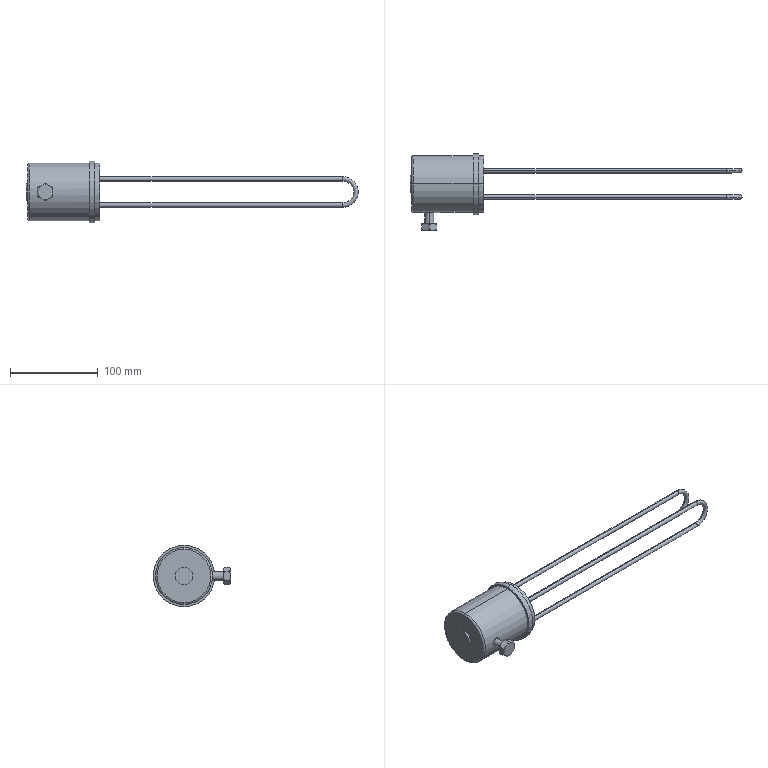Part | SolidWorks | features ICE 6, Chamfer 1, CirPattern 1, Fillet 1, MirrorPattern 1, Revolution 1, Sweep 1 | 1 solid | 41 faces | box 378 x 88 x 70 mm | volume 302343 mm3 | cylinder 18 | plane 13 | torus 6 | cone 4 | commonest cylinder face diameters 5 x8 65 x4 10 x2 20 x2 70 x2
STEP:
#1=CARTESIAN_POINT('',(282.5,-30.,2.5));
#2=VERTEX_POINT('',#1);
#3=CARTESIAN_POINT('',(282.5,-30.,-2.5));
#4=VERTEX_POINT('',#3);
#5=CARTESIAN_POINT('',(282.5,-30.,0.));
#6=DIRECTION('',(-1.,0.,0.));
#7=DIRECTION('',(0.,0.,-1.));
#8=AXIS2_PLACEMENT_3D('',#5,#6,#7);
#9=CIRCLE('',#8,2.5);
#10=EDGE_CURVE('',#2,#4,#9,.T.);
#11=ORIENTED_EDGE('',*,*,#10,.F.);
#12=CARTESIAN_POINT('',(282.5,-30.,-32.5));
#13=VERTEX_POINT('',#12);
#14=CARTESIAN_POINT('',(282.5,-30.,-15.));
#15=DIRECTION('',(0.,1.,0.));
#16=DIRECTION('',(0.,0.,1.));
#17=AXIS2_PLACEMENT_3D('',#14,#15,#16);
#18=CIRCLE('',#17,17.5);
#19=EDGE_CURVE('',#2,#13,#18,.T.);
#20=ORIENTED_EDGE('',*,*,#19,.T.);
#21=CARTESIAN_POINT('',(282.5,-30.,-27.5));
#22=VERTEX_POINT('',#21);
#23=CARTESIAN_POINT('',(282.5,-30.,-30.));
#24=DIRECTION('',(1.,0.,0.));
#25=DIRECTION('',(0.,0.,1.));
#26=AXIS2_PLACEMENT_3D('',#23,#24,#25);
#27=CIRCLE('',#26,2.5);
#28=EDGE_CURVE('',#13,#22,#27,.T.);
#29=ORIENTED_EDGE('',*,*,#28,.T.);
#30=CARTESIAN_POINT('',(282.5,-30.,-15.));
#31=DIRECTION('',(0.,1.,0.));
#32=DIRECTION('',(0.,0.,1.));
#33=AXIS2_PLACEMENT_3D('',#30,#31,#32);
#34=CIRCLE('',#33,12.5);
#35=EDGE_CURVE('',#4,#22,#34,.T.);
#36=ORIENTED_EDGE('',*,*,#35,.F.);
#37=EDGE_LOOP('',(#11,#20,#29,#36));
#38=FACE_OUTER_BOUND('',#37,.T.);
#39=CARTESIAN_POINT('',(282.5,-30.,-15.));
#40=DIRECTION('',(0.,1.,0.));
#41=DIRECTION('',(0.,0.,1.));
#42=AXIS2_PLACEMENT_3D('',#39,#40,#41);
#43=TOROIDAL_SURFACE('',#42,15.,2.5);
#44=ADVANCED_FACE('',(#38),#43,.T.);
#45=CARTESIAN_POINT('',(282.5,0.,-2.5));
#46=VERTEX_POINT('',#45);
#47=CARTESIAN_POINT('',(282.5,0.,2.5));
#48=VERTEX_POINT('',#47);
#49=CARTESIAN_POINT('',(282.5,0.,0.));
#50=DIRECTION('',(1.,0.,0.));
#51=DIRECTION('',(0.,0.,-1.));
#52=AXIS2_PLACEMENT_3D('',#49,#50,#51);
#53=CIRCLE('',#52,2.5);
#54=EDGE_CURVE('',#46,#48,#53,.T.);
#55=ORIENTED_EDGE('',*,*,#54,.T.);
#56=CARTESIAN_POINT('',(282.5,0.,-32.5));
#57=VERTEX_POINT('',#56);
#58=CARTESIAN_POINT('',(282.5,0.,-15.));
#59=DIRECTION('',(0.,1.,0.));
#60=DIRECTION('',(0.,0.,1.));
#61=AXIS2_PLACEMENT_3D('',#58,#59,#60);
#62=CIRCLE('',#61,17.5);
#63=EDGE_CURVE('',#48,#57,#62,.T.);
#64=ORIENTED_EDGE('',*,*,#63,.T.);
#65=CARTESIAN_POINT('',(282.5,0.,-27.5));
#66=VERTEX_POINT('',#65);
#67=CARTESIAN_POINT('',(282.5,0.,-30.));
#68=DIRECTION('',(-1.,0.,0.));
#69=DIRECTION('',(0.,0.,1.));
#70=AXIS2_PLACEMENT_3D('',#67,#68,#69);
#71=CIRCLE('',#70,2.5);
#72=EDGE_CURVE('',#66,#57,#71,.T.);
#73=ORIENTED_EDGE('',*,*,#72,.F.);
#74=CARTESIAN_POINT('',(282.5,0.,-15.));
#75=DIRECTION('',(0.,1.,0.));
#76=DIRECTION('',(0.,0.,1.));
#77=AXIS2_PLACEMENT_3D('',#74,#75,#76);
#78=CIRCLE('',#77,12.5);
#79=EDGE_CURVE('',#46,#66,#78,.T.);
#80=ORIENTED_EDGE('',*,*,#79,.F.);
#81=EDGE_LOOP('',(#55,#64,#73,#80));
#82=FACE_OUTER_BOUND('',#81,.T.);
#83=CARTESIAN_POINT('',(282.5,0.,-15.));
#84=DIRECTION('',(0.,1.,0.));
#85=DIRECTION('',(0.,0.,1.));
#86=AXIS2_PLACEMENT_3D('',#83,#84,#85);
#87=TOROIDAL_SURFACE('',#86,15.,2.5);
#88=ADVANCED_FACE('',(#82),#87,.T.);
#89=CARTESIAN_POINT('',(6.,-15.,17.5));
#90=VERTEX_POINT('',#89);
#91=CARTESIAN_POINT('',(6.,-15.,-47.5));
#92=VERTEX_POINT('',#91);
#93=CARTESIAN_POINT('',(6.,-15.,-15.));
#94=DIRECTION('',(-1.,0.,0.));
#95=DIRECTION('',(0.,0.,1.));
#96=AXIS2_PLACEMENT_3D('',#93,#94,#95);
#97=CIRCLE('',#96,32.5);
#98=EDGE_CURVE('',#90,#92,#97,.T.);
#99=ORIENTED_EDGE('',*,*,#98,.T.);
#100=CARTESIAN_POINT('',(0.,-15.,-47.5));
#101=VERTEX_POINT('',#100);
#102=CARTESIAN_POINT('',(6.,-15.,-47.5));
#103=DIRECTION('',(-1.,0.,0.));
#104=VECTOR('',#103,1000.);
#105=LINE('',#102,#104);
#106=EDGE_CURVE('',#92,#101,#105,.T.);
#107=ORIENTED_EDGE('',*,*,#106,.T.);
#108=CARTESIAN_POINT('',(0.,-15.,17.5));
#109=VERTEX_POINT('',#108);
#110=CARTESIAN_POINT('',(0.,-15.,-15.));
#111=DIRECTION('',(-1.,0.,0.));
#112=DIRECTION('',(0.,0.,1.));
#113=AXIS2_PLACEMENT_3D('',#110,#111,#112);
#114=CIRCLE('',#113,32.5);
#115=EDGE_CURVE('',#109,#101,#114,.T.);
#116=ORIENTED_EDGE('',*,*,#115,.F.);
#117=CARTESIAN_POINT('',(6.,-15.,17.5));
#118=DIRECTION('',(-1.,0.,0.));
#119=VECTOR('',#118,1000.);
#120=LINE('',#117,#119);
#121=EDGE_CURVE('',#90,#109,#120,.T.);
#122=ORIENTED_EDGE('',*,*,#121,.F.);
#123=EDGE_LOOP('',(#99,#107,#116,#122));
#124=FACE_OUTER_BOUND('',#123,.T.);
#125=CARTESIAN_POINT('',(6.,-15.,-15.));
#126=DIRECTION('',(-1.,0.,0.));
#127=DIRECTION('',(0.,0.,1.));
#128=AXIS2_PLACEMENT_3D('',#125,#126,#127);
#129=CYLINDRICAL_SURFACE('',#128,32.5);
#130=ADVANCED_FACE('',(#124),#129,.T.);
#131=ORIENTED_EDGE('',*,*,#10,.T.);
#132=CARTESIAN_POINT('',(6.,-30.,-2.5));
#133=VERTEX_POINT('',#132);
#134=CARTESIAN_POINT('',(282.5,-30.,-2.5));
#135=DIRECTION('',(-1.,0.,0.));
#136=VECTOR('',#135,1000.);
#137=LINE('',#134,#136);
#138=EDGE_CURVE('',#4,#133,#137,.T.);
#139=ORIENTED_EDGE('',*,*,#138,.T.);
#140=CARTESIAN_POINT('',(6.,-30.,2.5));
#141=VERTEX_POINT('',#140);
#142=CARTESIAN_POINT('',(6.,-30.,0.));
#143=DIRECTION('',(-1.,0.,0.));
#144=DIRECTION('',(0.,0.,1.));
#145=AXIS2_PLACEMENT_3D('',#142,#143,#144);
#146=CIRCLE('',#145,2.5);
#147=EDGE_CURVE('',#141,#133,#146,.T.);
#148=ORIENTED_EDGE('',*,*,#147,.F.);
#149=CARTESIAN_POINT('',(282.5,-30.,2.5));
#150=DIRECTION('',(-1.,0.,0.));
#151=VECTOR('',#150,1000.);
#152=LINE('',#149,#151);
#153=EDGE_CURVE('',#2,#141,#152,.T.);
#154=ORIENTED_EDGE('',*,*,#153,.F.);
#155=EDGE_LOOP('',(#131,#139,#148,#154));
#156=FACE_OUTER_BOUND('',#155,.T.);
#157=CARTESIAN_POINT('',(282.5,-30.,0.));
#158=DIRECTION('',(-1.,0.,0.));
#159=DIRECTION('',(0.,0.,1.));
#160=AXIS2_PLACEMENT_3D('',#157,#158,#159);
#161=CYLINDRICAL_SURFACE('',#160,2.5);
#162=ADVANCED_FACE('',(#156),#161,.T.);
#163=ORIENTED_EDGE('',*,*,#72,.T.);
#164=CARTESIAN_POINT('',(6.,0.,-32.5));
#165=VERTEX_POINT('',#164);
#166=CARTESIAN_POINT('',(282.5,0.,-32.5));
#167=DIRECTION('',(-1.,0.,0.));
#168=VECTOR('',#167,1000.);
#169=LINE('',#166,#168);
#170=EDGE_CURVE('',#57,#165,#169,.T.);
#171=ORIENTED_EDGE('',*,*,#170,.T.);
#172=CARTESIAN_POINT('',(6.,0.,-27.5));
#173=VERTEX_POINT('',#172);
#174=CARTESIAN_POINT('',(6.,0.,-30.));
#175=DIRECTION('',(1.,0.,0.));
#176=DIRECTION('',(0.,0.,1.));
#177=AXIS2_PLACEMENT_3D('',#174,#175,#176);
#178=CIRCLE('',#177,2.5);
#179=EDGE_CURVE('',#165,#173,#178,.T.);
#180=ORIENTED_EDGE('',*,*,#179,.T.);
#181=CARTESIAN_POINT('',(282.5,0.,-27.5));
#182=DIRECTION('',(-1.,0.,0.));
#183=VECTOR('',#182,1000.);
#184=LINE('',#181,#183);
#185=EDGE_CURVE('',#66,#173,#184,.T.);
#186=ORIENTED_EDGE('',*,*,#185,.F.);
#187=EDGE_LOOP('',(#163,#171,#180,#186));
#188=FACE_OUTER_BOUND('',#187,.T.);
#189=CARTESIAN_POINT('',(282.5,0.,-30.));
#190=DIRECTION('',(-1.,0.,0.));
#191=DIRECTION('',(0.,0.,1.));
#192=AXIS2_PLACEMENT_3D('',#189,#190,#191);
#193=CYLINDRICAL_SURFACE('',#192,2.5);
#194=ADVANCED_FACE('',(#188),#193,.T.);
#195=ORIENTED_EDGE('',*,*,#54,.F.);
#196=CARTESIAN_POINT('',(6.,0.,-2.5));
#197=VERTEX_POINT('',#196);
#198=CARTESIAN_POINT('',(282.5,0.,-2.5));
#199=DIRECTION('',(-1.,0.,0.));
#200=VECTOR('',#199,1000.);
#201=LINE('',#198,#200);
#202=EDGE_CURVE('',#46,#197,#201,.T.);
#203=ORIENTED_EDGE('',*,*,#202,.T.);
#204=CARTESIAN_POINT('',(6.,0.,2.5));
#205=VERTEX_POINT('',#204);
#206=CARTESIAN_POINT('',(6.,0.,0.));
#207=DIRECTION('',(-1.,0.,0.));
#208=DIRECTION('',(0.,0.,1.));
#209=AXIS2_PLACEMENT_3D('',#206,#207,#208);
#210=CIRCLE('',#209,2.5);
#211=EDGE_CURVE('',#205,#197,#210,.T.);
#212=ORIENTED_EDGE('',*,*,#211,.F.);
#213=CARTESIAN_POINT('',(282.5,0.,2.5));
#214=DIRECTION('',(-1.,0.,0.));
#215=VECTOR('',#214,1000.);
#216=LINE('',#213,#215);
#217=EDGE_CURVE('',#48,#205,#216,.T.);
#218=ORIENTED_EDGE('',*,*,#217,.F.);
#219=EDGE_LOOP('',(#195,#203,#212,#218));
#220=FACE_OUTER_BOUND('',#219,.T.);
#221=CARTESIAN_POINT('',(282.5,0.,0.));
#222=DIRECTION('',(-1.,0.,0.));
#223=DIRECTION('',(0.,0.,1.));
#224=AXIS2_PLACEMENT_3D('',#221,#222,#223);
#225=CYLINDRICAL_SURFACE('',#224,2.5);
#226=ADVANCED_FACE('',(#220),#225,.T.);
#227=ORIENTED_EDGE('',*,*,#28,.F.);
#228=CARTESIAN_POINT('',(6.,-30.,-32.5));
#229=VERTEX_POINT('',#228);
#230=CARTESIAN_POINT('',(282.5,-30.,-32.5));
#231=DIRECTION('',(-1.,0.,0.));
#232=VECTOR('',#231,1000.);
#233=LINE('',#230,#232);
#234=EDGE_CURVE('',#13,#229,#233,.T.);
#235=ORIENTED_EDGE('',*,*,#234,.T.);
#236=CARTESIAN_POINT('',(6.,-30.,-27.5));
#237=VERTEX_POINT('',#236);
#238=CARTESIAN_POINT('',(6.,-30.,-30.));
#239=DIRECTION('',(1.,0.,0.));
#240=DIRECTION('',(0.,0.,1.));
#241=AXIS2_PLACEMENT_3D('',#238,#239,#240);
#242=CIRCLE('',#241,2.5);
#243=EDGE_CURVE('',#229,#237,#242,.T.);
#244=ORIENTED_EDGE('',*,*,#243,.T.);
#245=CARTESIAN_POINT('',(282.5,-30.,-27.5));
#246=DIRECTION('',(-1.,0.,0.));
#247=VECTOR('',#246,1000.);
#248=LINE('',#245,#247);
#249=EDGE_CURVE('',#22,#237,#248,.T.);
#250=ORIENTED_EDGE('',*,*,#249,.F.);
#251=EDGE_LOOP('',(#227,#235,#244,#250));
#252=FACE_OUTER_BOUND('',#251,.T.);
#253=CARTESIAN_POINT('',(282.5,-30.,-30.));
#254=DIRECTION('',(-1.,0.,0.));
#255=DIRECTION('',(0.,0.,1.));
#256=AXIS2_PLACEMENT_3D('',#253,#254,#255);
#257=CYLINDRICAL_SURFACE('',#256,2.5);
#258=ADVANCED_FACE('',(#252),#257,.T.);
#259=CARTESIAN_POINT('',(0.,-15.,-50.));
#260=VERTEX_POINT('',#259);
#261=CARTESIAN_POINT('',(0.,-15.,20.));
#262=VERTEX_POINT('',#261);
#263=CARTESIAN_POINT('',(0.,-15.,-15.));
#264=DIRECTION('',(1.,0.,0.));
#265=DIRECTION('',(0.,0.,-1.));
#266=AXIS2_PLACEMENT_3D('',#263,#264,#265);
#267=CIRCLE('',#266,35.);
#268=EDGE_CURVE('',#260,#262,#267,.T.);
#269=ORIENTED_EDGE('',*,*,#268,.F.);
#270=CARTESIAN_POINT('',(-6.,-15.,-50.));
#271=VERTEX_POINT('',#270);
#272=CARTESIAN_POINT('',(300.,-15.,-50.));
#273=DIRECTION('',(-1.,0.,0.));
#274=VECTOR('',#273,1000.);
#275=LINE('',#272,#274);
#276=EDGE_CURVE('',#260,#271,#275,.T.);
#277=ORIENTED_EDGE('',*,*,#276,.T.);
#278=CARTESIAN_POINT('',(-6.,-15.,20.));
#279=VERTEX_POINT('',#278);
#280=CARTESIAN_POINT('',(-6.,-15.,-15.));
#281=DIRECTION('',(-1.,0.,0.));
#282=DIRECTION('',(0.,0.,1.));
#283=AXIS2_PLACEMENT_3D('',#280,#281,#282);
#284=CIRCLE('',#283,35.);
#285=EDGE_CURVE('',#279,#271,#284,.T.);
#286=ORIENTED_EDGE('',*,*,#285,.F.);
#287=CARTESIAN_POINT('',(300.,-15.,20.));
#288=DIRECTION('',(-1.,0.,0.));
#289=VECTOR('',#288,1000.);
#290=LINE('',#287,#289);
#291=EDGE_CURVE('',#262,#279,#290,.T.);
#292=ORIENTED_EDGE('',*,*,#291,.F.);
#293=EDGE_LOOP('',(#269,#277,#286,#292));
#294=FACE_OUTER_BOUND('',#293,.T.);
#295=CARTESIAN_POINT('',(300.,-15.,-15.));
#296=DIRECTION('',(-1.,0.,0.));
#297=DIRECTION('',(0.,0.,1.));
#298=AXIS2_PLACEMENT_3D('',#295,#296,#297);
#299=CYLINDRICAL_SURFACE('',#298,35.);
#300=ADVANCED_FACE('',(#294),#299,.T.);
#301=CARTESIAN_POINT('',(-74.,-15.,-47.5));
#302=VERTEX_POINT('',#301);
#303=CARTESIAN_POINT('',(-74.,-15.,17.5));
#304=VERTEX_POINT('',#303);
#305=CARTESIAN_POINT('',(-74.,-15.,-15.));
#306=DIRECTION('',(1.,0.,0.));
#307=DIRECTION('',(0.,0.,1.));
#308=AXIS2_PLACEMENT_3D('',#305,#306,#307);
#309=CIRCLE('',#308,32.5);
#310=EDGE_CURVE('',#302,#304,#309,.T.);
#311=ORIENTED_EDGE('',*,*,#310,.F.);
#312=CARTESIAN_POINT('',(-76.,-15.,-45.5));
#313=VERTEX_POINT('',#312);
#314=CARTESIAN_POINT('',(-74.,-15.,-45.5));
#315=DIRECTION('',(0.,1.,0.));
#316=DIRECTION('',(0.,0.,1.));
#317=AXIS2_PLACEMENT_3D('',#314,#315,#316);
#318=CIRCLE('',#317,2.);
#319=EDGE_CURVE('',#302,#313,#318,.T.);
#320=ORIENTED_EDGE('',*,*,#319,.T.);
#321=CARTESIAN_POINT('',(-76.,-15.,15.5));
#322=VERTEX_POINT('',#321);
#323=CARTESIAN_POINT('',(-76.,-15.,-15.));
#324=DIRECTION('',(-1.,0.,0.));
#325=DIRECTION('',(0.,0.,1.));
#326=AXIS2_PLACEMENT_3D('',#323,#324,#325);
#327=CIRCLE('',#326,30.5);
#328=EDGE_CURVE('',#322,#313,#327,.T.);
#329=ORIENTED_EDGE('',*,*,#328,.F.);
#330=CARTESIAN_POINT('',(-74.,-15.,15.5));
#331=DIRECTION('',(0.,-1.,0.));
#332=DIRECTION('',(0.,0.,-1.));
#333=AXIS2_PLACEMENT_3D('',#330,#331,#332);
#334=CIRCLE('',#333,2.);
#335=EDGE_CURVE('',#304,#322,#334,.T.);
#336=ORIENTED_EDGE('',*,*,#335,.F.);
#337=EDGE_LOOP('',(#311,#320,#329,#336));
#338=FACE_OUTER_BOUND('',#337,.T.);
#339=CARTESIAN_POINT('',(-74.,-15.,-15.));
#340=DIRECTION('',(-1.,0.,0.));
#341=DIRECTION('',(0.,0.,1.));
#342=AXIS2_PLACEMENT_3D('',#339,#340,#341);
#343=TOROIDAL_SURFACE('',#342,30.5,2.);
#344=ADVANCED_FACE('',(#338),#343,.T.);
#345=CARTESIAN_POINT('',(-56.,-60.,-10.));
#346=VERTEX_POINT('',#345);
#347=CARTESIAN_POINT('',(-56.,-60.,-20.));
#348=VERTEX_POINT('',#347);
#349=CARTESIAN_POINT('',(-56.,-60.,-15.));
#350=DIRECTION('',(0.,1.,0.));
#351=DIRECTION('',(0.,0.,-1.));
#352=AXIS2_PLACEMENT_3D('',#349,#350,#351);
#353=CIRCLE('',#352,5.);
#354=EDGE_CURVE('',#346,#348,#353,.T.);
#355=ORIENTED_EDGE('',*,*,#354,.T.);
#356=CARTESIAN_POINT('',(-56.,-47.113,-20.));
#357=VERTEX_POINT('',#356);
#358=CARTESIAN_POINT('',(-56.,-60.,-20.));
#359=DIRECTION('',(0.,1.,0.));
#360=VECTOR('',#359,1000.);
#361=LINE('',#358,#360);
#362=EDGE_CURVE('',#348,#357,#361,.T.);
#363=ORIENTED_EDGE('',*,*,#362,.T.);
#364=CARTESIAN_POINT('',(-56.,-47.113,-10.));
#365=VERTEX_POINT('',#364);
#366=CARTESIAN_POINT('',(-56.,-47.113,-20.));
#367=CARTESIAN_POINT('',(-55.674,-47.113,-20.));
#368=CARTESIAN_POINT('',(-55.349,-47.118,-19.968));
#369=CARTESIAN_POINT('',(-54.702,-47.138,-19.84));
#370=CARTESIAN_POINT('',(-54.387,-47.152,-19.744));
#371=CARTESIAN_POINT('',(-53.786,-47.188,-19.495));
#372=CARTESIAN_POINT('',(-53.494,-47.21,-19.339));
#373=CARTESIAN_POINT('',(-52.949,-47.257,-18.975));
#374=CARTESIAN_POINT('',(-52.697,-47.282,-18.768));
#375=CARTESIAN_POINT('',(-52.236,-47.332,-18.308));
#376=CARTESIAN_POINT('',(-52.025,-47.358,-18.051));
#377=CARTESIAN_POINT('',(-51.663,-47.404,-17.509));
#378=CARTESIAN_POINT('',(-51.509,-47.425,-17.222));
#379=CARTESIAN_POINT('',(-51.32,-47.452,-16.767));
#380=CARTESIAN_POINT('',(-51.264,-47.46,-16.611));
#381=CARTESIAN_POINT('',(-51.168,-47.474,-16.297));
#382=CARTESIAN_POINT('',(-51.129,-47.48,-16.139));
#383=CARTESIAN_POINT('',(-51.033,-47.495,-15.66));
#384=CARTESIAN_POINT('',(-51.,-47.5,-15.334));
#385=CARTESIAN_POINT('',(-51.,-47.5,-14.673));
#386=CARTESIAN_POINT('',(-51.032,-47.495,-14.348));
#387=CARTESIAN_POINT('',(-51.159,-47.476,-13.708));
#388=CARTESIAN_POINT('',(-51.255,-47.461,-13.39));
#389=CARTESIAN_POINT('',(-51.506,-47.426,-12.785));
#390=CARTESIAN_POINT('',(-51.659,-47.405,-12.498));
#391=CARTESIAN_POINT('',(-52.022,-47.358,-11.954));
#392=CARTESIAN_POINT('',(-52.232,-47.333,-11.697));
#393=CARTESIAN_POINT('',(-52.692,-47.282,-11.237));
#394=CARTESIAN_POINT('',(-52.943,-47.257,-11.029));
#395=CARTESIAN_POINT('',(-53.49,-47.21,-10.663));
#396=CARTESIAN_POINT('',(-53.779,-47.188,-10.508));
#397=CARTESIAN_POINT('',(-54.381,-47.152,-10.258));
#398=CARTESIAN_POINT('',(-54.696,-47.138,-10.162));
#399=CARTESIAN_POINT('',(-55.342,-47.118,-10.033));
#400=CARTESIAN_POINT('',(-55.669,-47.113,-10.));
#401=CARTESIAN_POINT('',(-56.,-47.113,-10.));
#402=B_SPLINE_CURVE_WITH_KNOTS('',3,(#366,#367,#368,#369,#370,#371,#372,#373,#374,#375,#376,#377,#378,#379,#380,#381,#382,#383,#384,#385,#386,#387,#388,#389,#390,#391,#392,#393,#394,#395,#396,#397,#398,#399,#400,#401),.UNSPECIFIED.,.F.,.F.,(4,2,2,2,2,2,2,2,2,2,2,2,2,2,2,2,2,4),(0.01566,0.01663,0.01761,0.01859,0.01957,0.02055,0.02152,0.02201,0.0225,0.02348,0.02446,0.02544,0.02642,0.02739,0.02837,0.02935,0.03033,0.03131),.UNSPECIFIED.);
#403=EDGE_CURVE('',#357,#365,#402,.T.);
#404=ORIENTED_EDGE('',*,*,#403,.T.);
#405=CARTESIAN_POINT('',(-56.,-60.,-10.));
#406=DIRECTION('',(0.,1.,0.));
#407=VECTOR('',#406,1000.);
#408=LINE('',#405,#407);
#409=EDGE_CURVE('',#346,#365,#408,.T.);
#410=ORIENTED_EDGE('',*,*,#409,.F.);
#411=EDGE_LOOP('',(#355,#363,#404,#410));
#412=FACE_OUTER_BOUND('',#411,.T.);
#413=CARTESIAN_POINT('',(-56.,-60.,-15.));
#414=DIRECTION('',(0.,1.,0.));
#415=DIRECTION('',(0.,0.,1.));
#416=AXIS2_PLACEMENT_3D('',#413,#414,#415);
#417=CYLINDRICAL_SURFACE('',#416,5.);
#418=ADVANCED_FACE('',(#412),#417,.T.);
#419=CARTESIAN_POINT('',(-76.,-15.,-5.));
#420=VERTEX_POINT('',#419);
#421=CARTESIAN_POINT('',(-76.,-15.,-25.));
#422=VERTEX_POINT('',#421);
#423=CARTESIAN_POINT('',(-76.,-15.,-15.));
#424=DIRECTION('',(-1.,0.,0.));
#425=DIRECTION('',(0.,0.,1.));
#426=AXIS2_PLACEMENT_3D('',#423,#424,#425);
#427=CIRCLE('',#426,10.);
#428=EDGE_CURVE('',#420,#422,#427,.T.);
#429=ORIENTED_EDGE('',*,*,#428,.T.);
#430=CARTESIAN_POINT('',(-78.,-15.,-25.));
#431=VERTEX_POINT('',#430);
#432=CARTESIAN_POINT('',(-78.,-15.,-25.));
#433=DIRECTION('',(-1.,0.,0.));
#434=VECTOR('',#433,1000.);
#435=LINE('',#432,#434);
#436=EDGE_CURVE('',#422,#431,#435,.T.);
#437=ORIENTED_EDGE('',*,*,#436,.T.);
#438=CARTESIAN_POINT('',(-78.,-15.,-5.));
#439=VERTEX_POINT('',#438);
#440=CARTESIAN_POINT('',(-78.,-15.,-15.));
#441=DIRECTION('',(-1.,0.,0.));
#442=DIRECTION('',(0.,0.,1.));
#443=AXIS2_PLACEMENT_3D('',#440,#441,#442);
#444=CIRCLE('',#443,10.);
#445=EDGE_CURVE('',#439,#431,#444,.T.);
#446=ORIENTED_EDGE('',*,*,#445,.F.);
#447=CARTESIAN_POINT('',(-78.,-15.,-5.));
#448=DIRECTION('',(-1.,0.,0.));
#449=VECTOR('',#448,1000.);
#450=LINE('',#447,#449);
#451=EDGE_CURVE('',#420,#439,#450,.T.);
#452=ORIENTED_EDGE('',*,*,#451,.F.);
#453=EDGE_LOOP('',(#429,#437,#446,#452));
#454=FACE_OUTER_BOUND('',#453,.T.);
#455=CARTESIAN_POINT('',(-78.,-15.,-15.));
#456=DIRECTION('',(-1.,0.,0.));
#457=DIRECTION('',(0.,0.,1.));
#458=AXIS2_PLACEMENT_3D('',#455,#456,#457);
#459=CYLINDRICAL_SURFACE('',#458,10.);
#460=ADVANCED_FACE('',(#454),#459,.T.);
#461=CARTESIAN_POINT('',(-6.,-15.,17.5));
#462=VERTEX_POINT('',#461);
#463=CARTESIAN_POINT('',(-6.,-15.,-47.5));
#464=VERTEX_POINT('',#463);
#465=CARTESIAN_POINT('',(-6.,-15.,-15.));
#466=DIRECTION('',(-1.,0.,0.));
#467=DIRECTION('',(0.,0.,1.));
#468=AXIS2_PLACEMENT_3D('',#465,#466,#467);
#469=CIRCLE('',#468,32.5);
#470=EDGE_CURVE('',#462,#464,#469,.T.);
#471=ORIENTED_EDGE('',*,*,#470,.T.);
#472=CARTESIAN_POINT('',(-78.,-15.,-47.5));
#473=DIRECTION('',(-1.,0.,0.));
#474=VECTOR('',#473,1000.);
#475=LINE('',#472,#474);
#476=EDGE_CURVE('',#464,#302,#475,.T.);
#477=ORIENTED_EDGE('',*,*,#476,.T.);
#478=ORIENTED_EDGE('',*,*,#310,.T.);
#479=CARTESIAN_POINT('',(-78.,-15.,17.5));
#480=DIRECTION('',(-1.,0.,0.));
#481=VECTOR('',#480,1000.);
#482=LINE('',#479,#481);
#483=EDGE_CURVE('',#462,#304,#482,.T.);
#484=ORIENTED_EDGE('',*,*,#483,.F.);
#485=EDGE_LOOP('',(#471,#477,#478,#484));
#486=FACE_OUTER_BOUND('',#485,.T.);
#487=CARTESIAN_POINT('',(-78.,-15.,-15.));
#488=DIRECTION('',(-1.,0.,0.));
#489=DIRECTION('',(0.,0.,1.));
#490=AXIS2_PLACEMENT_3D('',#487,#488,#489);
#491=CYLINDRICAL_SURFACE('',#490,32.5);
#492=ADVANCED_FACE('',(#486),#491,.T.);
#493=CARTESIAN_POINT('',(-56.,-68.,-23.5));
#494=VERTEX_POINT('',#493);
#495=CARTESIAN_POINT('',(-56.,-68.,-6.5));
#496=VERTEX_POINT('',#495);
#497=CARTESIAN_POINT('',(-56.,-68.,-15.));
#498=DIRECTION('',(0.,-1.,0.));
#499=DIRECTION('',(0.,0.,-1.));
#500=AXIS2_PLACEMENT_3D('',#497,#498,#499);
#501=CIRCLE('',#500,8.5);
#502=EDGE_CURVE('',#494,#496,#501,.T.);
#503=ORIENTED_EDGE('',*,*,#502,.F.);
#504=CARTESIAN_POINT('',(-56.,-66.5,-25.));
#505=VERTEX_POINT('',#504);
#506=CARTESIAN_POINT('',(-56.,-68.,-23.5));
#507=DIRECTION('',(0.,0.7071,-0.7071));
#508=VECTOR('',#507,1000.);
#509=LINE('',#506,#508);
#510=EDGE_CURVE('',#494,#505,#509,.T.);
#511=ORIENTED_EDGE('',*,*,#510,.T.);
#512=CARTESIAN_POINT('',(-47.34,-66.5,-20.));
#513=VERTEX_POINT('',#512);
#514=CARTESIAN_POINT('',(-56.,-66.5,-25.));
#515=CARTESIAN_POINT('',(-55.323,-66.891,-24.609));
#516=CARTESIAN_POINT('',(-54.631,-67.223,-24.21));
#517=CARTESIAN_POINT('',(-53.556,-67.579,-23.589));
#518=CARTESIAN_POINT('',(-53.192,-67.673,-23.379));
#519=CARTESIAN_POINT('',(-52.447,-67.804,-22.949));
#520=CARTESIAN_POINT('',(-52.064,-67.839,-22.727));
#521=CARTESIAN_POINT('',(-50.93,-67.842,-22.073));
#522=CARTESIAN_POINT('',(-50.187,-67.709,-21.644));
#523=CARTESIAN_POINT('',(-48.721,-67.23,-20.798));
#524=CARTESIAN_POINT('',(-48.02,-66.893,-20.393));
#525=CARTESIAN_POINT('',(-47.34,-66.5,-20.));
#526=B_SPLINE_CURVE_WITH_KNOTS('',3,(#514,#515,#516,#517,#518,#519,#520,#521,#522,#523,#524,#525),.UNSPECIFIED.,.F.,.F.,(4,2,2,2,2,4),(0.000000254,0.002583,0.003874,0.005165,0.007747,0.01033),.UNSPECIFIED.);
#527=EDGE_CURVE('',#505,#513,#526,.T.);
#528=ORIENTED_EDGE('',*,*,#527,.T.);
#529=CARTESIAN_POINT('',(-47.34,-66.5,-10.));
#530=VERTEX_POINT('',#529);
#531=CARTESIAN_POINT('',(-47.34,-66.5,-20.));
#532=CARTESIAN_POINT('',(-47.34,-66.694,-19.612));
#533=CARTESIAN_POINT('',(-47.34,-66.875,-19.217));
#534=CARTESIAN_POINT('',(-47.34,-67.202,-18.404));
#535=CARTESIAN_POINT('',(-47.34,-67.347,-17.991));
#536=CARTESIAN_POINT('',(-47.34,-67.584,-17.156));
#537=CARTESIAN_POINT('',(-47.34,-67.678,-16.733));
#538=CARTESIAN_POINT('',(-47.34,-67.806,-15.875));
#539=CARTESIAN_POINT('',(-47.34,-67.84,-15.437));
#540=CARTESIAN_POINT('',(-47.34,-67.84,-14.119));
#541=CARTESIAN_POINT('',(-47.34,-67.704,-13.263));
#542=CARTESIAN_POINT('',(-47.34,-67.346,-12.006));
#543=CARTESIAN_POINT('',(-47.34,-67.2,-11.59));
#544=CARTESIAN_POINT('',(-47.34,-66.874,-10.781));
#545=CARTESIAN_POINT('',(-47.34,-66.693,-10.387));
#546=CARTESIAN_POINT('',(-47.34,-66.5,-10.));
#547=B_SPLINE_CURVE_WITH_KNOTS('',3,(#531,#532,#533,#534,#535,#536,#537,#538,#539,#540,#541,#542,#543,#544,#545,#546),.UNSPECIFIED.,.F.,.F.,(4,2,2,2,2,2,2,4),(0.006413,0.007709,0.009005,0.0103,0.0116,0.01419,0.01548,0.01678),.UNSPECIFIED.);
#548=EDGE_CURVE('',#513,#530,#547,.T.);
#549=ORIENTED_EDGE('',*,*,#548,.T.);
#550=CARTESIAN_POINT('',(-56.,-66.5,-5.));
#551=VERTEX_POINT('',#550);
#552=CARTESIAN_POINT('',(-47.34,-66.5,-10.));
#553=CARTESIAN_POINT('',(-48.016,-66.891,-9.609));
#554=CARTESIAN_POINT('',(-48.708,-67.223,-9.21));
#555=CARTESIAN_POINT('',(-49.783,-67.579,-8.589));
#556=CARTESIAN_POINT('',(-50.148,-67.673,-8.379));
#557=CARTESIAN_POINT('',(-50.892,-67.804,-7.949));
#558=CARTESIAN_POINT('',(-51.276,-67.839,-7.727));
#559=CARTESIAN_POINT('',(-52.41,-67.842,-7.073));
#560=CARTESIAN_POINT('',(-53.153,-67.709,-6.644));
#561=CARTESIAN_POINT('',(-54.619,-67.23,-5.798));
#562=CARTESIAN_POINT('',(-55.319,-66.893,-5.393));
#563=CARTESIAN_POINT('',(-56.,-66.5,-5.));
#564=B_SPLINE_CURVE_WITH_KNOTS('',3,(#552,#553,#554,#555,#556,#557,#558,#559,#560,#561,#562,#563),.UNSPECIFIED.,.F.,.F.,(4,2,2,2,2,4),(0.000000254,0.002583,0.003874,0.005165,0.007747,0.01033),.UNSPECIFIED.);
#565=EDGE_CURVE('',#530,#551,#564,.T.);
#566=ORIENTED_EDGE('',*,*,#565,.T.);
#567=CARTESIAN_POINT('',(-56.,-68.,-6.5));
#568=DIRECTION('',(0.,0.7071,0.7071));
#569=VECTOR('',#568,1000.);
#570=LINE('',#567,#569);
#571=EDGE_CURVE('',#496,#551,#570,.T.);
#572=ORIENTED_EDGE('',*,*,#571,.F.);
#573=EDGE_LOOP('',(#503,#511,#528,#549,#566,#572));
#574=FACE_OUTER_BOUND('',#573,.T.);
#575=CARTESIAN_POINT('',(-56.,-68.,-15.));
#576=DIRECTION('',(0.,1.,0.));
#577=DIRECTION('',(0.,0.,1.));
#578=AXIS2_PLACEMENT_3D('',#575,#576,#577);
#579=CONICAL_SURFACE('',#578,8.5,0.7854);
#580=ADVANCED_FACE('',(#574),#579,.T.);
#581=CARTESIAN_POINT('',(-56.,-60.,-6.5));
#582=VERTEX_POINT('',#581);
#583=CARTESIAN_POINT('',(-56.,-60.,-23.5));
#584=VERTEX_POINT('',#583);
#585=CARTESIAN_POINT('',(-56.,-60.,-15.));
#586=DIRECTION('',(0.,1.,0.));
#587=DIRECTION('',(0.,0.,-1.));
#588=AXIS2_PLACEMENT_3D('',#585,#586,#587);
#589=CIRCLE('',#588,8.5);
#590=EDGE_CURVE('',#582,#584,#589,.T.);
#591=ORIENTED_EDGE('',*,*,#590,.F.);
#592=CARTESIAN_POINT('',(-56.,-61.5,-5.));
#593=VERTEX_POINT('',#592);
#594=CARTESIAN_POINT('',(-56.,-61.5,-5.));
#595=DIRECTION('',(0.,-0.7071,0.7071));
#596=VECTOR('',#595,1000.);
#597=LINE('',#594,#596);
#598=EDGE_CURVE('',#582,#593,#597,.T.);
#599=ORIENTED_EDGE('',*,*,#598,.T.);
#600=CARTESIAN_POINT('',(-47.34,-61.5,-10.));
#601=VERTEX_POINT('',#600);
#602=CARTESIAN_POINT('',(-56.,-61.5,-5.));
#603=CARTESIAN_POINT('',(-55.323,-61.109,-5.391));
#604=CARTESIAN_POINT('',(-54.631,-60.777,-5.79));
#605=CARTESIAN_POINT('',(-53.556,-60.421,-6.411));
#606=CARTESIAN_POINT('',(-53.192,-60.327,-6.621));
#607=CARTESIAN_POINT('',(-52.447,-60.196,-7.051));
#608=CARTESIAN_POINT('',(-52.064,-60.161,-7.273));
#609=CARTESIAN_POINT('',(-50.93,-60.158,-7.927));
#610=CARTESIAN_POINT('',(-50.187,-60.291,-8.356));
#611=CARTESIAN_POINT('',(-48.721,-60.77,-9.202));
#612=CARTESIAN_POINT('',(-48.02,-61.107,-9.607));
#613=CARTESIAN_POINT('',(-47.34,-61.5,-10.));
#614=B_SPLINE_CURVE_WITH_KNOTS('',3,(#602,#603,#604,#605,#606,#607,#608,#609,#610,#611,#612,#613),.UNSPECIFIED.,.F.,.F.,(4,2,2,2,2,4),(0.000000254,0.002583,0.003874,0.005165,0.007747,0.01033),.UNSPECIFIED.);
#615=EDGE_CURVE('',#593,#601,#614,.T.);
#616=ORIENTED_EDGE('',*,*,#615,.T.);
#617=CARTESIAN_POINT('',(-47.34,-61.5,-20.));
#618=VERTEX_POINT('',#617);
#619=CARTESIAN_POINT('',(-47.34,-61.5,-10.));
#620=CARTESIAN_POINT('',(-47.34,-61.307,-10.387));
#621=CARTESIAN_POINT('',(-47.34,-61.126,-10.781));
#622=CARTESIAN_POINT('',(-47.34,-60.8,-11.59));
#623=CARTESIAN_POINT('',(-47.34,-60.654,-12.006));
#624=CARTESIAN_POINT('',(-47.34,-60.296,-13.263));
#625=CARTESIAN_POINT('',(-47.34,-60.16,-14.119));
#626=CARTESIAN_POINT('',(-47.34,-60.16,-15.437));
#627=CARTESIAN_POINT('',(-47.34,-60.194,-15.875));
#628=CARTESIAN_POINT('',(-47.34,-60.322,-16.733));
#629=CARTESIAN_POINT('',(-47.34,-60.416,-17.156));
#630=CARTESIAN_POINT('',(-47.34,-60.653,-17.991));
#631=CARTESIAN_POINT('',(-47.34,-60.798,-18.404));
#632=CARTESIAN_POINT('',(-47.34,-61.125,-19.217));
#633=CARTESIAN_POINT('',(-47.34,-61.306,-19.612));
#634=CARTESIAN_POINT('',(-47.34,-61.5,-20.));
#635=B_SPLINE_CURVE_WITH_KNOTS('',3,(#619,#620,#621,#622,#623,#624,#625,#626,#627,#628,#629,#630,#631,#632,#633,#634),.UNSPECIFIED.,.F.,.F.,(4,2,2,2,2,2,2,4),(0.005329,0.006624,0.007919,0.01051,0.0118,0.0131,0.01439,0.01569),.UNSPECIFIED.);
#636=EDGE_CURVE('',#601,#618,#635,.T.);
#637=ORIENTED_EDGE('',*,*,#636,.T.);
#638=CARTESIAN_POINT('',(-56.,-61.5,-25.));
#639=VERTEX_POINT('',#638);
#640=CARTESIAN_POINT('',(-47.34,-61.5,-20.));
#641=CARTESIAN_POINT('',(-48.016,-61.109,-20.391));
#642=CARTESIAN_POINT('',(-48.708,-60.777,-20.79));
#643=CARTESIAN_POINT('',(-49.783,-60.421,-21.411));
#644=CARTESIAN_POINT('',(-50.148,-60.327,-21.621));
#645=CARTESIAN_POINT('',(-50.892,-60.196,-22.051));
#646=CARTESIAN_POINT('',(-51.276,-60.161,-22.273));
#647=CARTESIAN_POINT('',(-52.41,-60.158,-22.927));
#648=CARTESIAN_POINT('',(-53.153,-60.291,-23.356));
#649=CARTESIAN_POINT('',(-54.619,-60.77,-24.202));
#650=CARTESIAN_POINT('',(-55.319,-61.107,-24.607));
#651=CARTESIAN_POINT('',(-56.,-61.5,-25.));
#652=B_SPLINE_CURVE_WITH_KNOTS('',3,(#640,#641,#642,#643,#644,#645,#646,#647,#648,#649,#650,#651),.UNSPECIFIED.,.F.,.F.,(4,2,2,2,2,4),(0.000000254,0.002583,0.003874,0.005165,0.007747,0.01033),.UNSPECIFIED.);
#653=EDGE_CURVE('',#618,#639,#652,.T.);
#654=ORIENTED_EDGE('',*,*,#653,.T.);
#655=CARTESIAN_POINT('',(-56.,-61.5,-25.));
#656=DIRECTION('',(0.,-0.7071,-0.7071));
#657=VECTOR('',#656,1000.);
#658=LINE('',#655,#657);
#659=EDGE_CURVE('',#584,#639,#658,.T.);
#660=ORIENTED_EDGE('',*,*,#659,.F.);
#661=EDGE_LOOP('',(#591,#599,#616,#637,#654,#660));
#662=FACE_OUTER_BOUND('',#661,.T.);
#663=CARTESIAN_POINT('',(-56.,-61.5,-15.));
#664=DIRECTION('',(0.,-1.,0.));
#665=DIRECTION('',(0.,0.,-1.));
#666=AXIS2_PLACEMENT_3D('',#663,#664,#665);
#667=CONICAL_SURFACE('',#666,10.,0.7854);
#668=ADVANCED_FACE('',(#662),#667,.T.);
#669=ORIENTED_EDGE('',*,*,#470,.F.);
#670=CARTESIAN_POINT('',(-6.,-15.,-15.));
#671=DIRECTION('',(-1.,0.,0.));
#672=DIRECTION('',(0.,0.,1.));
#673=AXIS2_PLACEMENT_3D('',#670,#671,#672);
#674=CIRCLE('',#673,32.5);
#675=EDGE_CURVE('',#464,#462,#674,.T.);
#676=ORIENTED_EDGE('',*,*,#675,.F.);
#677=EDGE_LOOP('',(#669,#676));
#678=FACE_BOUND('',#677,.T.);
#679=ORIENTED_EDGE('',*,*,#285,.T.);
#680=CARTESIAN_POINT('',(-6.,-15.,-15.));
#681=DIRECTION('',(-1.,0.,0.));
#682=DIRECTION('',(0.,0.,1.));
#683=AXIS2_PLACEMENT_3D('',#680,#681,#682);
#684=CIRCLE('',#683,35.);
#685=EDGE_CURVE('',#271,#279,#684,.T.);
#686=ORIENTED_EDGE('',*,*,#685,.T.);
#687=EDGE_LOOP('',(#679,#686));
#688=FACE_OUTER_BOUND('',#687,.T.);
#689=CARTESIAN_POINT('',(-6.,-15.,42.5));
#690=DIRECTION('',(-1.,0.,0.));
#691=DIRECTION('',(0.,0.,1.));
#692=AXIS2_PLACEMENT_3D('',#689,#690,#691);
#693=PLANE('',#692);
#694=ADVANCED_FACE('',(#678,#688),#693,.T.);
#695=ORIENTED_EDGE('',*,*,#598,.F.);
#696=CARTESIAN_POINT('',(-56.,-60.,-15.));
#697=DIRECTION('',(0.,1.,0.));
#698=DIRECTION('',(0.,0.,-1.));
#699=AXIS2_PLACEMENT_3D('',#696,#697,#698);
#700=CIRCLE('',#699,8.5);
#701=EDGE_CURVE('',#584,#582,#700,.T.);
#702=ORIENTED_EDGE('',*,*,#701,.F.);
#703=ORIENTED_EDGE('',*,*,#659,.T.);
#704=CARTESIAN_POINT('',(-64.66,-61.5,-20.));
#705=VERTEX_POINT('',#704);
#706=CARTESIAN_POINT('',(-56.,-61.5,-25.));
#707=CARTESIAN_POINT('',(-56.677,-61.109,-24.609));
#708=CARTESIAN_POINT('',(-57.369,-60.777,-24.21));
#709=CARTESIAN_POINT('',(-58.444,-60.421,-23.589));
#710=CARTESIAN_POINT('',(-58.808,-60.327,-23.379));
#711=CARTESIAN_POINT('',(-59.553,-60.196,-22.949));
#712=CARTESIAN_POINT('',(-59.936,-60.161,-22.727));
#713=CARTESIAN_POINT('',(-61.07,-60.158,-22.073));
#714=CARTESIAN_POINT('',(-61.813,-60.291,-21.644));
#715=CARTESIAN_POINT('',(-63.279,-60.77,-20.798));
#716=CARTESIAN_POINT('',(-63.98,-61.107,-20.393));
#717=CARTESIAN_POINT('',(-64.66,-61.5,-20.));
#718=B_SPLINE_CURVE_WITH_KNOTS('',3,(#706,#707,#708,#709,#710,#711,#712,#713,#714,#715,#716,#717),.UNSPECIFIED.,.F.,.F.,(4,2,2,2,2,4),(0.000000254,0.002583,0.003874,0.005165,0.007747,0.01033),.UNSPECIFIED.);
#719=EDGE_CURVE('',#639,#705,#718,.T.);
#720=ORIENTED_EDGE('',*,*,#719,.T.);
#721=CARTESIAN_POINT('',(-64.66,-61.5,-10.));
#722=VERTEX_POINT('',#721);
#723=CARTESIAN_POINT('',(-64.66,-61.5,-20.));
#724=CARTESIAN_POINT('',(-64.66,-61.306,-19.612));
#725=CARTESIAN_POINT('',(-64.66,-61.125,-19.217));
#726=CARTESIAN_POINT('',(-64.66,-60.798,-18.404));
#727=CARTESIAN_POINT('',(-64.66,-60.653,-17.991));
#728=CARTESIAN_POINT('',(-64.66,-60.416,-17.156));
#729=CARTESIAN_POINT('',(-64.66,-60.322,-16.733));
#730=CARTESIAN_POINT('',(-64.66,-60.194,-15.875));
#731=CARTESIAN_POINT('',(-64.66,-60.16,-15.437));
#732=CARTESIAN_POINT('',(-64.66,-60.16,-14.119));
#733=CARTESIAN_POINT('',(-64.66,-60.296,-13.263));
#734=CARTESIAN_POINT('',(-64.66,-60.654,-12.006));
#735=CARTESIAN_POINT('',(-64.66,-60.8,-11.59));
#736=CARTESIAN_POINT('',(-64.66,-61.126,-10.781));
#737=CARTESIAN_POINT('',(-64.66,-61.307,-10.387));
#738=CARTESIAN_POINT('',(-64.66,-61.5,-10.));
#739=B_SPLINE_CURVE_WITH_KNOTS('',3,(#723,#724,#725,#726,#727,#728,#729,#730,#731,#732,#733,#734,#735,#736,#737,#738),.UNSPECIFIED.,.F.,.F.,(4,2,2,2,2,2,2,4),(0.006413,0.007709,0.009005,0.0103,0.0116,0.01419,0.01548,0.01678),.UNSPECIFIED.);
#740=EDGE_CURVE('',#705,#722,#739,.T.);
#741=ORIENTED_EDGE('',*,*,#740,.T.);
#742=CARTESIAN_POINT('',(-64.66,-61.5,-10.));
#743=CARTESIAN_POINT('',(-63.984,-61.109,-9.609));
#744=CARTESIAN_POINT('',(-63.292,-60.777,-9.21));
#745=CARTESIAN_POINT('',(-62.217,-60.421,-8.589));
#746=CARTESIAN_POINT('',(-61.852,-60.327,-8.379));
#747=CARTESIAN_POINT('',(-61.108,-60.196,-7.949));
#748=CARTESIAN_POINT('',(-60.724,-60.161,-7.727));
#749=CARTESIAN_POINT('',(-59.59,-60.158,-7.073));
#750=CARTESIAN_POINT('',(-58.847,-60.291,-6.644));
#751=CARTESIAN_POINT('',(-57.381,-60.77,-5.798));
#752=CARTESIAN_POINT('',(-56.681,-61.107,-5.393));
#753=CARTESIAN_POINT('',(-56.,-61.5,-5.));
#754=B_SPLINE_CURVE_WITH_KNOTS('',3,(#742,#743,#744,#745,#746,#747,#748,#749,#750,#751,#752,#753),.UNSPECIFIED.,.F.,.F.,(4,2,2,2,2,4),(0.000000254,0.002583,0.003874,0.005165,0.007747,0.01033),.UNSPECIFIED.);
#755=EDGE_CURVE('',#722,#593,#754,.T.);
#756=ORIENTED_EDGE('',*,*,#755,.T.);
#757=EDGE_LOOP('',(#695,#702,#703,#720,#741,#756));
#758=FACE_OUTER_BOUND('',#757,.T.);
#759=CARTESIAN_POINT('',(-56.,-61.5,-15.));
#760=DIRECTION('',(0.,-1.,0.));
#761=DIRECTION('',(0.,0.,-1.));
#762=AXIS2_PLACEMENT_3D('',#759,#760,#761);
#763=CONICAL_SURFACE('',#762,10.,0.7854);
#764=ADVANCED_FACE('',(#758),#763,.T.);
#765=ORIENTED_EDGE('',*,*,#510,.F.);
#766=CARTESIAN_POINT('',(-56.,-68.,-15.));
#767=DIRECTION('',(0.,-1.,0.));
#768=DIRECTION('',(0.,0.,-1.));
#769=AXIS2_PLACEMENT_3D('',#766,#767,#768);
#770=CIRCLE('',#769,8.5);
#771=EDGE_CURVE('',#496,#494,#770,.T.);
#772=ORIENTED_EDGE('',*,*,#771,.F.);
#773=ORIENTED_EDGE('',*,*,#571,.T.);
#774=CARTESIAN_POINT('',(-64.66,-66.5,-10.));
#775=VERTEX_POINT('',#774);
#776=CARTESIAN_POINT('',(-56.,-66.5,-5.));
#777=CARTESIAN_POINT('',(-56.677,-66.891,-5.391));
#778=CARTESIAN_POINT('',(-57.369,-67.223,-5.79));
#779=CARTESIAN_POINT('',(-58.444,-67.579,-6.411));
#780=CARTESIAN_POINT('',(-58.808,-67.673,-6.621));
#781=CARTESIAN_POINT('',(-59.553,-67.804,-7.051));
#782=CARTESIAN_POINT('',(-59.936,-67.839,-7.273));
#783=CARTESIAN_POINT('',(-61.07,-67.842,-7.927));
#784=CARTESIAN_POINT('',(-61.813,-67.709,-8.356));
#785=CARTESIAN_POINT('',(-63.279,-67.23,-9.202));
#786=CARTESIAN_POINT('',(-63.98,-66.893,-9.607));
#787=CARTESIAN_POINT('',(-64.66,-66.5,-10.));
#788=B_SPLINE_CURVE_WITH_KNOTS('',3,(#776,#777,#778,#779,#780,#781,#782,#783,#784,#785,#786,#787),.UNSPECIFIED.,.F.,.F.,(4,2,2,2,2,4),(0.000000254,0.002583,0.003874,0.005165,0.007747,0.01033),.UNSPECIFIED.);
#789=EDGE_CURVE('',#551,#775,#788,.T.);
#790=ORIENTED_EDGE('',*,*,#789,.T.);
#791=CARTESIAN_POINT('',(-64.66,-66.5,-20.));
#792=VERTEX_POINT('',#791);
#793=CARTESIAN_POINT('',(-64.66,-66.5,-10.));
#794=CARTESIAN_POINT('',(-64.66,-66.693,-10.387));
#795=CARTESIAN_POINT('',(-64.66,-66.874,-10.781));
#796=CARTESIAN_POINT('',(-64.66,-67.2,-11.59));
#797=CARTESIAN_POINT('',(-64.66,-67.346,-12.006));
#798=CARTESIAN_POINT('',(-64.66,-67.704,-13.263));
#799=CARTESIAN_POINT('',(-64.66,-67.84,-14.119));
#800=CARTESIAN_POINT('',(-64.66,-67.84,-15.437));
#801=CARTESIAN_POINT('',(-64.66,-67.806,-15.875));
#802=CARTESIAN_POINT('',(-64.66,-67.678,-16.733));
#803=CARTESIAN_POINT('',(-64.66,-67.584,-17.156));
#804=CARTESIAN_POINT('',(-64.66,-67.347,-17.991));
#805=CARTESIAN_POINT('',(-64.66,-67.202,-18.404));
#806=CARTESIAN_POINT('',(-64.66,-66.875,-19.217));
#807=CARTESIAN_POINT('',(-64.66,-66.694,-19.612));
#808=CARTESIAN_POINT('',(-64.66,-66.5,-20.));
#809=B_SPLINE_CURVE_WITH_KNOTS('',3,(#793,#794,#795,#796,#797,#798,#799,#800,#801,#802,#803,#804,#805,#806,#807,#808),.UNSPECIFIED.,.F.,.F.,(4,2,2,2,2,2,2,4),(0.005329,0.006624,0.007919,0.01051,0.0118,0.0131,0.01439,0.01569),.UNSPECIFIED.);
#810=EDGE_CURVE('',#775,#792,#809,.T.);
#811=ORIENTED_EDGE('',*,*,#810,.T.);
#812=CARTESIAN_POINT('',(-64.66,-66.5,-20.));
#813=CARTESIAN_POINT('',(-63.984,-66.891,-20.391));
#814=CARTESIAN_POINT('',(-63.292,-67.223,-20.79));
#815=CARTESIAN_POINT('',(-62.217,-67.579,-21.411));
#816=CARTESIAN_POINT('',(-61.852,-67.673,-21.621));
#817=CARTESIAN_POINT('',(-61.108,-67.804,-22.051));
#818=CARTESIAN_POINT('',(-60.724,-67.839,-22.273));
#819=CARTESIAN_POINT('',(-59.59,-67.842,-22.927));
#820=CARTESIAN_POINT('',(-58.847,-67.709,-23.356));
#821=CARTESIAN_POINT('',(-57.381,-67.23,-24.202));
#822=CARTESIAN_POINT('',(-56.681,-66.893,-24.607));
#823=CARTESIAN_POINT('',(-56.,-66.5,-25.));
#824=B_SPLINE_CURVE_WITH_KNOTS('',3,(#812,#813,#814,#815,#816,#817,#818,#819,#820,#821,#822,#823),.UNSPECIFIED.,.F.,.F.,(4,2,2,2,2,4),(0.000000254,0.002583,0.003874,0.005165,0.007747,0.01033),.UNSPECIFIED.);
#825=EDGE_CURVE('',#792,#505,#824,.T.);
#826=ORIENTED_EDGE('',*,*,#825,.T.);
#827=EDGE_LOOP('',(#765,#772,#773,#790,#811,#826));
#828=FACE_OUTER_BOUND('',#827,.T.);
#829=CARTESIAN_POINT('',(-56.,-68.,-15.));
#830=DIRECTION('',(0.,1.,0.));
#831=DIRECTION('',(0.,0.,1.));
#832=AXIS2_PLACEMENT_3D('',#829,#830,#831);
#833=CONICAL_SURFACE('',#832,8.5,0.7854);
#834=ADVANCED_FACE('',(#828),#833,.T.);
#835=ORIENTED_EDGE('',*,*,#476,.F.);
#836=ORIENTED_EDGE('',*,*,#675,.T.);
#837=ORIENTED_EDGE('',*,*,#483,.T.);
#838=CARTESIAN_POINT('',(-74.,-15.,-15.));
#839=DIRECTION('',(1.,0.,0.));
#840=DIRECTION('',(0.,0.,1.));
#841=AXIS2_PLACEMENT_3D('',#838,#839,#840);
#842=CIRCLE('',#841,32.5);
#843=EDGE_CURVE('',#304,#302,#842,.T.);
#844=ORIENTED_EDGE('',*,*,#843,.T.);
#845=EDGE_LOOP('',(#835,#836,#837,#844));
#846=FACE_OUTER_BOUND('',#845,.T.);
#847=CARTESIAN_POINT('',(-56.,-47.113,-10.));
#848=CARTESIAN_POINT('',(-56.331,-47.113,-10.));
#849=CARTESIAN_POINT('',(-56.656,-47.118,-10.033));
#850=CARTESIAN_POINT('',(-57.136,-47.133,-10.128));
#851=CARTESIAN_POINT('',(-57.295,-47.139,-10.168));
#852=CARTESIAN_POINT('',(-57.609,-47.153,-10.263));
#853=CARTESIAN_POINT('',(-57.765,-47.161,-10.319));
#854=CARTESIAN_POINT('',(-58.219,-47.188,-10.507));
#855=CARTESIAN_POINT('',(-58.506,-47.21,-10.661));
#856=CARTESIAN_POINT('',(-59.049,-47.256,-11.024));
#857=CARTESIAN_POINT('',(-59.306,-47.282,-11.235));
#858=CARTESIAN_POINT('',(-59.766,-47.332,-11.696));
#859=CARTESIAN_POINT('',(-59.973,-47.357,-11.947));
#860=CARTESIAN_POINT('',(-60.339,-47.404,-12.493));
#861=CARTESIAN_POINT('',(-60.494,-47.426,-12.784));
#862=CARTESIAN_POINT('',(-60.743,-47.461,-13.385));
#863=CARTESIAN_POINT('',(-60.84,-47.476,-13.701));
#864=CARTESIAN_POINT('',(-60.968,-47.495,-14.347));
#865=CARTESIAN_POINT('',(-61.,-47.5,-14.671));
#866=CARTESIAN_POINT('',(-61.,-47.5,-15.325));
#867=CARTESIAN_POINT('',(-60.967,-47.495,-15.657));
#868=CARTESIAN_POINT('',(-60.84,-47.476,-16.298));
#869=CARTESIAN_POINT('',(-60.745,-47.462,-16.61));
#870=CARTESIAN_POINT('',(-60.557,-47.435,-17.065));
#871=CARTESIAN_POINT('',(-60.486,-47.425,-17.215));
#872=CARTESIAN_POINT('',(-60.331,-47.404,-17.504));
#873=CARTESIAN_POINT('',(-60.247,-47.393,-17.644));
#874=CARTESIAN_POINT('',(-59.976,-47.358,-18.05));
#875=CARTESIAN_POINT('',(-59.769,-47.333,-18.302));
#876=CARTESIAN_POINT('',(-59.303,-47.282,-18.768));
#877=CARTESIAN_POINT('',(-59.051,-47.257,-18.975));
#878=CARTESIAN_POINT('',(-58.51,-47.21,-19.337));
#879=CARTESIAN_POINT('',(-58.217,-47.188,-19.494));
#880=CARTESIAN_POINT('',(-57.612,-47.152,-19.744));
#881=CARTESIAN_POINT('',(-57.3,-47.138,-19.839));
#882=CARTESIAN_POINT('',(-56.658,-47.118,-19.967));
#883=CARTESIAN_POINT('',(-56.327,-47.113,-20.));
#884=CARTESIAN_POINT('',(-56.,-47.113,-20.));
#885=B_SPLINE_CURVE_WITH_KNOTS('',3,(#847,#848,#849,#850,#851,#852,#853,#854,#855,#856,#857,#858,#859,#860,#861,#862,#863,#864,#865,#866,#867,#868,#869,#870,#871,#872,#873,#874,#875,#876,#877,#878,#879,#880,#881,#882,#883,#884),.UNSPECIFIED.,.F.,.F.,(4,2,2,2,2,2,2,2,2,2,2,2,2,2,2,2,2,2,4),(0.,0.0009785,0.001468,0.001957,0.002935,0.003914,0.004892,0.005871,0.006849,0.007828,0.008806,0.009785,0.01027,0.01076,0.01174,0.01272,0.0137,0.01468,0.01566),.UNSPECIFIED.);
#886=EDGE_CURVE('',#365,#357,#885,.T.);
#887=ORIENTED_EDGE('',*,*,#886,.F.);
#888=ORIENTED_EDGE('',*,*,#403,.F.);
#889=EDGE_LOOP('',(#887,#888));
#890=FACE_BOUND('',#889,.T.);
#891=CARTESIAN_POINT('',(-78.,-15.,-15.));
#892=DIRECTION('',(-1.,0.,0.));
#893=DIRECTION('',(0.,0.,1.));
#894=AXIS2_PLACEMENT_3D('',#891,#892,#893);
#895=CYLINDRICAL_SURFACE('',#894,32.5);
#896=ADVANCED_FACE('',(#846,#890),#895,.T.);
#897=ORIENTED_EDGE('',*,*,#328,.T.);
#898=CARTESIAN_POINT('',(-76.,-15.,-15.));
#899=DIRECTION('',(-1.,0.,0.));
#900=DIRECTION('',(0.,0.,1.));
#901=AXIS2_PLACEMENT_3D('',#898,#899,#900);
#902=CIRCLE('',#901,30.5);
#903=EDGE_CURVE('',#313,#322,#902,.T.);
#904=ORIENTED_EDGE('',*,*,#903,.T.);
#905=EDGE_LOOP('',(#897,#904));
#906=FACE_OUTER_BOUND('',#905,.T.);
#907=ORIENTED_EDGE('',*,*,#428,.F.);
#908=CARTESIAN_POINT('',(-76.,-15.,-15.));
#909=DIRECTION('',(-1.,0.,0.));
#910=DIRECTION('',(0.,0.,1.));
#911=AXIS2_PLACEMENT_3D('',#908,#909,#910);
#912=CIRCLE('',#911,10.);
#913=EDGE_CURVE('',#422,#420,#912,.T.);
#914=ORIENTED_EDGE('',*,*,#913,.F.);
#915=EDGE_LOOP('',(#907,#914));
#916=FACE_BOUND('',#915,.T.);
#917=CARTESIAN_POINT('',(-76.,-15.,17.5));
#918=DIRECTION('',(-1.,0.,0.));
#919=DIRECTION('',(0.,0.,1.));
#920=AXIS2_PLACEMENT_3D('',#917,#918,#919);
#921=PLANE('',#920);
#922=ADVANCED_FACE('',(#906,#916),#921,.T.);
#923=ORIENTED_EDGE('',*,*,#436,.F.);
#924=ORIENTED_EDGE('',*,*,#913,.T.);
#925=ORIENTED_EDGE('',*,*,#451,.T.);
#926=CARTESIAN_POINT('',(-78.,-15.,-15.));
#927=DIRECTION('',(-1.,0.,0.));
#928=DIRECTION('',(0.,0.,1.));
#929=AXIS2_PLACEMENT_3D('',#926,#927,#928);
#930=CIRCLE('',#929,10.);
#931=EDGE_CURVE('',#431,#439,#930,.T.);
#932=ORIENTED_EDGE('',*,*,#931,.F.);
#933=EDGE_LOOP('',(#923,#924,#925,#932));
#934=FACE_OUTER_BOUND('',#933,.T.);
#935=CARTESIAN_POINT('',(-78.,-15.,-15.));
#936=DIRECTION('',(-1.,0.,0.));
#937=DIRECTION('',(0.,0.,1.));
#938=AXIS2_PLACEMENT_3D('',#935,#936,#937);
#939=CYLINDRICAL_SURFACE('',#938,10.);
#940=ADVANCED_FACE('',(#934),#939,.T.);
#941=ORIENTED_EDGE('',*,*,#445,.T.);
#942=ORIENTED_EDGE('',*,*,#931,.T.);
#943=EDGE_LOOP('',(#941,#942));
#944=FACE_OUTER_BOUND('',#943,.T.);
#945=CARTESIAN_POINT('',(-78.,-15.,-5.));
#946=DIRECTION('',(-1.,0.,0.));
#947=DIRECTION('',(0.,0.,1.));
#948=AXIS2_PLACEMENT_3D('',#945,#946,#947);
#949=PLANE('',#948);
#950=ADVANCED_FACE('',(#944),#949,.T.);
#951=ORIENTED_EDGE('',*,*,#362,.F.);
#952=CARTESIAN_POINT('',(-56.,-60.,-15.));
#953=DIRECTION('',(0.,1.,0.));
#954=DIRECTION('',(0.,0.,-1.));
#955=AXIS2_PLACEMENT_3D('',#952,#953,#954);
#956=CIRCLE('',#955,5.);
#957=EDGE_CURVE('',#348,#346,#956,.T.);
#958=ORIENTED_EDGE('',*,*,#957,.T.);
#959=ORIENTED_EDGE('',*,*,#409,.T.);
#960=ORIENTED_EDGE('',*,*,#886,.T.);
#961=EDGE_LOOP('',(#951,#958,#959,#960));
#962=FACE_OUTER_BOUND('',#961,.T.);
#963=CARTESIAN_POINT('',(-56.,-60.,-15.));
#964=DIRECTION('',(0.,1.,0.));
#965=DIRECTION('',(0.,0.,1.));
#966=AXIS2_PLACEMENT_3D('',#963,#964,#965);
#967=CYLINDRICAL_SURFACE('',#966,5.);
#968=ADVANCED_FACE('',(#962),#967,.T.);
#969=ORIENTED_EDGE('',*,*,#771,.T.);
#970=ORIENTED_EDGE('',*,*,#502,.T.);
#971=EDGE_LOOP('',(#969,#970));
#972=FACE_OUTER_BOUND('',#971,.T.);
#973=CARTESIAN_POINT('',(-56.,-68.,-15.));
#974=DIRECTION('',(0.,-1.,0.));
#975=DIRECTION('',(0.,0.,-1.));
#976=AXIS2_PLACEMENT_3D('',#973,#974,#975);
#977=PLANE('',#976);
#978=ADVANCED_FACE('',(#972),#977,.T.);
#979=ORIENTED_EDGE('',*,*,#701,.T.);
#980=ORIENTED_EDGE('',*,*,#590,.T.);
#981=EDGE_LOOP('',(#979,#980));
#982=FACE_OUTER_BOUND('',#981,.T.);
#983=ORIENTED_EDGE('',*,*,#354,.F.);
#984=ORIENTED_EDGE('',*,*,#957,.F.);
#985=EDGE_LOOP('',(#983,#984));
#986=FACE_BOUND('',#985,.T.);
#987=CARTESIAN_POINT('',(-56.,-60.,-15.));
#988=DIRECTION('',(0.,-1.,0.));
#989=DIRECTION('',(0.,0.,-1.));
#990=AXIS2_PLACEMENT_3D('',#987,#988,#989);
#991=PLANE('',#990);
#992=ADVANCED_FACE('',(#982,#986),#991,.F.);
#993=CARTESIAN_POINT('',(-64.66,-60.,-20.));
#994=DIRECTION('',(0.,-1.,0.));
#995=VECTOR('',#994,1000.);
#996=LINE('',#993,#995);
#997=EDGE_CURVE('',#705,#792,#996,.T.);
#998=ORIENTED_EDGE('',*,*,#997,.T.);
#999=ORIENTED_EDGE('',*,*,#810,.F.);
#1000=CARTESIAN_POINT('',(-64.66,-60.,-10.));
#1001=DIRECTION('',(0.,-1.,0.));
#1002=VECTOR('',#1001,1000.);
#1003=LINE('',#1000,#1002);
#1004=EDGE_CURVE('',#722,#775,#1003,.T.);
#1005=ORIENTED_EDGE('',*,*,#1004,.F.);
#1006=ORIENTED_EDGE('',*,*,#740,.F.);
#1007=EDGE_LOOP('',(#998,#999,#1005,#1006));
#1008=FACE_OUTER_BOUND('',#1007,.T.);
#1009=CARTESIAN_POINT('',(-64.66,-60.,0.));
#1010=DIRECTION('',(-1.,0.,0.));
#1011=DIRECTION('',(0.,0.,1.));
#1012=AXIS2_PLACEMENT_3D('',#1009,#1010,#1011);
#1013=PLANE('',#1012);
#1014=ADVANCED_FACE('',(#1008),#1013,.T.);
#1015=ORIENTED_EDGE('',*,*,#1004,.T.);
#1016=ORIENTED_EDGE('',*,*,#789,.F.);
#1017=CARTESIAN_POINT('',(-56.,-60.,-5.));
#1018=DIRECTION('',(0.,-1.,0.));
#1019=VECTOR('',#1018,1000.);
#1020=LINE('',#1017,#1019);
#1021=EDGE_CURVE('',#593,#551,#1020,.T.);
#1022=ORIENTED_EDGE('',*,*,#1021,.F.);
#1023=ORIENTED_EDGE('',*,*,#755,.F.);
#1024=EDGE_LOOP('',(#1015,#1016,#1022,#1023));
#1025=FACE_OUTER_BOUND('',#1024,.T.);
#1026=CARTESIAN_POINT('',(-11.835,-60.,20.499));
#1027=DIRECTION('',(-0.5,0.,0.866));
#1028=DIRECTION('',(0.866,0.,0.5));
#1029=AXIS2_PLACEMENT_3D('',#1026,#1027,#1028);
#1030=PLANE('',#1029);
#1031=ADVANCED_FACE('',(#1025),#1030,.T.);
#1032=ORIENTED_EDGE('',*,*,#1021,.T.);
#1033=ORIENTED_EDGE('',*,*,#565,.F.);
#1034=CARTESIAN_POINT('',(-47.34,-60.,-10.));
#1035=DIRECTION('',(0.,-1.,0.));
#1036=VECTOR('',#1035,1000.);
#1037=LINE('',#1034,#1036);
#1038=EDGE_CURVE('',#601,#530,#1037,.T.);
#1039=ORIENTED_EDGE('',*,*,#1038,.F.);
#1040=ORIENTED_EDGE('',*,*,#615,.F.);
#1041=EDGE_LOOP('',(#1032,#1033,#1039,#1040));
#1042=FACE_OUTER_BOUND('',#1041,.T.);
#1043=CARTESIAN_POINT('',(-16.165,-60.,-27.999));
#1044=DIRECTION('',(0.5,0.,0.866));
#1045=DIRECTION('',(0.866,0.,-0.5));
#1046=AXIS2_PLACEMENT_3D('',#1043,#1044,#1045);
#1047=PLANE('',#1046);
#1048=ADVANCED_FACE('',(#1042),#1047,.T.);
#1049=ORIENTED_EDGE('',*,*,#1038,.T.);
#1050=ORIENTED_EDGE('',*,*,#548,.F.);
#1051=CARTESIAN_POINT('',(-47.34,-60.,-20.));
#1052=DIRECTION('',(0.,-1.,0.));
#1053=VECTOR('',#1052,1000.);
#1054=LINE('',#1051,#1053);
#1055=EDGE_CURVE('',#618,#513,#1054,.T.);
#1056=ORIENTED_EDGE('',*,*,#1055,.F.);
#1057=ORIENTED_EDGE('',*,*,#636,.F.);
#1058=EDGE_LOOP('',(#1049,#1050,#1056,#1057));
#1059=FACE_OUTER_BOUND('',#1058,.T.);
#1060=CARTESIAN_POINT('',(-47.34,-60.,0.));
#1061=DIRECTION('',(1.,0.,0.));
#1062=DIRECTION('',(0.,0.,-1.));
#1063=AXIS2_PLACEMENT_3D('',#1060,#1061,#1062);
#1064=PLANE('',#1063);
#1065=ADVANCED_FACE('',(#1059),#1064,.T.);
#1066=ORIENTED_EDGE('',*,*,#1055,.T.);
#1067=ORIENTED_EDGE('',*,*,#527,.F.);
#1068=CARTESIAN_POINT('',(-56.,-60.,-25.));
#1069=DIRECTION('',(0.,-1.,0.));
#1070=VECTOR('',#1069,1000.);
#1071=LINE('',#1068,#1070);
#1072=EDGE_CURVE('',#639,#505,#1071,.T.);
#1073=ORIENTED_EDGE('',*,*,#1072,.F.);
#1074=ORIENTED_EDGE('',*,*,#653,.F.);
#1075=EDGE_LOOP('',(#1066,#1067,#1073,#1074));
#1076=FACE_OUTER_BOUND('',#1075,.T.);
#1077=CARTESIAN_POINT('',(-3.175,-60.,5.499));
#1078=DIRECTION('',(0.5,0.,-0.866));
#1079=DIRECTION('',(-0.866,0.,-0.5));
#1080=AXIS2_PLACEMENT_3D('',#1077,#1078,#1079);
#1081=PLANE('',#1080);
#1082=ADVANCED_FACE('',(#1076),#1081,.T.);
#1083=ORIENTED_EDGE('',*,*,#1072,.T.);
#1084=ORIENTED_EDGE('',*,*,#825,.F.);
#1085=ORIENTED_EDGE('',*,*,#997,.F.);
#1086=ORIENTED_EDGE('',*,*,#719,.F.);
#1087=EDGE_LOOP('',(#1083,#1084,#1085,#1086));
#1088=FACE_OUTER_BOUND('',#1087,.T.);
#1089=CARTESIAN_POINT('',(-24.825,-60.,-42.999));
#1090=DIRECTION('',(-0.5,0.,-0.866));
#1091=DIRECTION('',(-0.866,0.,0.5));
#1092=AXIS2_PLACEMENT_3D('',#1089,#1090,#1091);
#1093=PLANE('',#1092);
#1094=ADVANCED_FACE('',(#1088),#1093,.T.);
#1095=ORIENTED_EDGE('',*,*,#319,.F.);
#1096=ORIENTED_EDGE('',*,*,#843,.F.);
#1097=ORIENTED_EDGE('',*,*,#335,.T.);
#1098=ORIENTED_EDGE('',*,*,#903,.F.);
#1099=EDGE_LOOP('',(#1095,#1096,#1097,#1098));
#1100=FACE_OUTER_BOUND('',#1099,.T.);
#1101=CARTESIAN_POINT('',(-74.,-15.,-15.));
#1102=DIRECTION('',(-1.,0.,0.));
#1103=DIRECTION('',(0.,0.,1.));
#1104=AXIS2_PLACEMENT_3D('',#1101,#1102,#1103);
#1105=TOROIDAL_SURFACE('',#1104,30.5,2.);
#1106=ADVANCED_FACE('',(#1100),#1105,.T.);
#1107=ORIENTED_EDGE('',*,*,#276,.F.);
#1108=CARTESIAN_POINT('',(0.,-15.,-15.));
#1109=DIRECTION('',(1.,0.,0.));
#1110=DIRECTION('',(0.,0.,-1.));
#1111=AXIS2_PLACEMENT_3D('',#1108,#1109,#1110);
#1112=CIRCLE('',#1111,35.);
#1113=EDGE_CURVE('',#262,#260,#1112,.T.);
#1114=ORIENTED_EDGE('',*,*,#1113,.F.);
#1115=ORIENTED_EDGE('',*,*,#291,.T.);
#1116=ORIENTED_EDGE('',*,*,#685,.F.);
#1117=EDGE_LOOP('',(#1107,#1114,#1115,#1116));
#1118=FACE_OUTER_BOUND('',#1117,.T.);
#1119=CARTESIAN_POINT('',(300.,-15.,-15.));
#1120=DIRECTION('',(-1.,0.,0.));
#1121=DIRECTION('',(0.,0.,1.));
#1122=AXIS2_PLACEMENT_3D('',#1119,#1120,#1121);
#1123=CYLINDRICAL_SURFACE('',#1122,35.);
#1124=ADVANCED_FACE('',(#1118),#1123,.T.);
#1125=ORIENTED_EDGE('',*,*,#63,.F.);
#1126=CARTESIAN_POINT('',(282.5,0.,0.));
#1127=DIRECTION('',(1.,0.,0.));
#1128=DIRECTION('',(0.,0.,-1.));
#1129=AXIS2_PLACEMENT_3D('',#1126,#1127,#1128);
#1130=CIRCLE('',#1129,2.5);
#1131=EDGE_CURVE('',#48,#46,#1130,.T.);
#1132=ORIENTED_EDGE('',*,*,#1131,.T.);
#1133=ORIENTED_EDGE('',*,*,#79,.T.);
#1134=CARTESIAN_POINT('',(282.5,0.,-30.));
#1135=DIRECTION('',(-1.,0.,0.));
#1136=DIRECTION('',(0.,0.,1.));
#1137=AXIS2_PLACEMENT_3D('',#1134,#1135,#1136);
#1138=CIRCLE('',#1137,2.5);
#1139=EDGE_CURVE('',#57,#66,#1138,.T.);
#1140=ORIENTED_EDGE('',*,*,#1139,.F.);
#1141=EDGE_LOOP('',(#1125,#1132,#1133,#1140));
#1142=FACE_OUTER_BOUND('',#1141,.T.);
#1143=CARTESIAN_POINT('',(282.5,0.,-15.));
#1144=DIRECTION('',(0.,1.,0.));
#1145=DIRECTION('',(0.,0.,1.));
#1146=AXIS2_PLACEMENT_3D('',#1143,#1144,#1145);
#1147=TOROIDAL_SURFACE('',#1146,15.,2.5);
#1148=ADVANCED_FACE('',(#1142),#1147,.T.);
#1149=ORIENTED_EDGE('',*,*,#19,.F.);
#1150=CARTESIAN_POINT('',(282.5,-30.,0.));
#1151=DIRECTION('',(-1.,0.,0.));
#1152=DIRECTION('',(0.,0.,-1.));
#1153=AXIS2_PLACEMENT_3D('',#1150,#1151,#1152);
#1154=CIRCLE('',#1153,2.5);
#1155=EDGE_CURVE('',#4,#2,#1154,.T.);
#1156=ORIENTED_EDGE('',*,*,#1155,.F.);
#1157=ORIENTED_EDGE('',*,*,#35,.T.);
#1158=CARTESIAN_POINT('',(282.5,-30.,-30.));
#1159=DIRECTION('',(1.,0.,0.));
#1160=DIRECTION('',(0.,0.,1.));
#1161=AXIS2_PLACEMENT_3D('',#1158,#1159,#1160);
#1162=CIRCLE('',#1161,2.5);
#1163=EDGE_CURVE('',#22,#13,#1162,.T.);
#1164=ORIENTED_EDGE('',*,*,#1163,.T.);
#1165=EDGE_LOOP('',(#1149,#1156,#1157,#1164));
#1166=FACE_OUTER_BOUND('',#1165,.T.);
#1167=CARTESIAN_POINT('',(282.5,-30.,-15.));
#1168=DIRECTION('',(0.,1.,0.));
#1169=DIRECTION('',(0.,0.,1.));
#1170=AXIS2_PLACEMENT_3D('',#1167,#1168,#1169);
#1171=TOROIDAL_SURFACE('',#1170,15.,2.5);
#1172=ADVANCED_FACE('',(#1166),#1171,.T.);
#1173=ORIENTED_EDGE('',*,*,#234,.F.);
#1174=ORIENTED_EDGE('',*,*,#1163,.F.);
#1175=ORIENTED_EDGE('',*,*,#249,.T.);
#1176=CARTESIAN_POINT('',(6.,-30.,-30.));
#1177=DIRECTION('',(1.,0.,0.));
#1178=DIRECTION('',(0.,0.,1.));
#1179=AXIS2_PLACEMENT_3D('',#1176,#1177,#1178);
#1180=CIRCLE('',#1179,2.5);
#1181=EDGE_CURVE('',#237,#229,#1180,.T.);
#1182=ORIENTED_EDGE('',*,*,#1181,.T.);
#1183=EDGE_LOOP('',(#1173,#1174,#1175,#1182));
#1184=FACE_OUTER_BOUND('',#1183,.T.);
#1185=CARTESIAN_POINT('',(282.5,-30.,-30.));
#1186=DIRECTION('',(-1.,0.,0.));
#1187=DIRECTION('',(0.,0.,1.));
#1188=AXIS2_PLACEMENT_3D('',#1185,#1186,#1187);
#1189=CYLINDRICAL_SURFACE('',#1188,2.5);
#1190=ADVANCED_FACE('',(#1184),#1189,.T.);
#1191=ORIENTED_EDGE('',*,*,#202,.F.);
#1192=ORIENTED_EDGE('',*,*,#1131,.F.);
#1193=ORIENTED_EDGE('',*,*,#217,.T.);
#1194=CARTESIAN_POINT('',(6.,0.,0.));
#1195=DIRECTION('',(-1.,0.,0.));
#1196=DIRECTION('',(0.,0.,1.));
#1197=AXIS2_PLACEMENT_3D('',#1194,#1195,#1196);
#1198=CIRCLE('',#1197,2.5);
#1199=EDGE_CURVE('',#197,#205,#1198,.T.);
#1200=ORIENTED_EDGE('',*,*,#1199,.F.);
#1201=EDGE_LOOP('',(#1191,#1192,#1193,#1200));
#1202=FACE_OUTER_BOUND('',#1201,.T.);
#1203=CARTESIAN_POINT('',(282.5,0.,0.));
#1204=DIRECTION('',(-1.,0.,0.));
#1205=DIRECTION('',(0.,0.,1.));
#1206=AXIS2_PLACEMENT_3D('',#1203,#1204,#1205);
#1207=CYLINDRICAL_SURFACE('',#1206,2.5);
#1208=ADVANCED_FACE('',(#1202),#1207,.T.);
#1209=ORIENTED_EDGE('',*,*,#170,.F.);
#1210=ORIENTED_EDGE('',*,*,#1139,.T.);
#1211=ORIENTED_EDGE('',*,*,#185,.T.);
#1212=CARTESIAN_POINT('',(6.,0.,-30.));
#1213=DIRECTION('',(1.,0.,0.));
#1214=DIRECTION('',(0.,0.,1.));
#1215=AXIS2_PLACEMENT_3D('',#1212,#1213,#1214);
#1216=CIRCLE('',#1215,2.5);
#1217=EDGE_CURVE('',#173,#165,#1216,.T.);
#1218=ORIENTED_EDGE('',*,*,#1217,.T.);
#1219=EDGE_LOOP('',(#1209,#1210,#1211,#1218));
#1220=FACE_OUTER_BOUND('',#1219,.T.);
#1221=CARTESIAN_POINT('',(282.5,0.,-30.));
#1222=DIRECTION('',(-1.,0.,0.));
#1223=DIRECTION('',(0.,0.,1.));
#1224=AXIS2_PLACEMENT_3D('',#1221,#1222,#1223);
#1225=CYLINDRICAL_SURFACE('',#1224,2.5);
#1226=ADVANCED_FACE('',(#1220),#1225,.T.);
#1227=ORIENTED_EDGE('',*,*,#138,.F.);
#1228=ORIENTED_EDGE('',*,*,#1155,.T.);
#1229=ORIENTED_EDGE('',*,*,#153,.T.);
#1230=CARTESIAN_POINT('',(6.,-30.,0.));
#1231=DIRECTION('',(-1.,0.,0.));
#1232=DIRECTION('',(0.,0.,1.));
#1233=AXIS2_PLACEMENT_3D('',#1230,#1231,#1232);
#1234=CIRCLE('',#1233,2.5);
#1235=EDGE_CURVE('',#133,#141,#1234,.T.);
#1236=ORIENTED_EDGE('',*,*,#1235,.F.);
#1237=EDGE_LOOP('',(#1227,#1228,#1229,#1236));
#1238=FACE_OUTER_BOUND('',#1237,.T.);
#1239=CARTESIAN_POINT('',(282.5,-30.,0.));
#1240=DIRECTION('',(-1.,0.,0.));
#1241=DIRECTION('',(0.,0.,1.));
#1242=AXIS2_PLACEMENT_3D('',#1239,#1240,#1241);
#1243=CYLINDRICAL_SURFACE('',#1242,2.5);
#1244=ADVANCED_FACE('',(#1238),#1243,.T.);
#1245=ORIENTED_EDGE('',*,*,#147,.T.);
#1246=ORIENTED_EDGE('',*,*,#1235,.T.);
#1247=EDGE_LOOP('',(#1245,#1246));
#1248=FACE_BOUND('',#1247,.T.);
#1249=ORIENTED_EDGE('',*,*,#1217,.F.);
#1250=ORIENTED_EDGE('',*,*,#179,.F.);
#1251=EDGE_LOOP('',(#1249,#1250));
#1252=FACE_BOUND('',#1251,.T.);
#1253=ORIENTED_EDGE('',*,*,#98,.F.);
#1254=CARTESIAN_POINT('',(6.,-15.,-15.));
#1255=DIRECTION('',(-1.,0.,0.));
#1256=DIRECTION('',(0.,0.,1.));
#1257=AXIS2_PLACEMENT_3D('',#1254,#1255,#1256);
#1258=CIRCLE('',#1257,32.5);
#1259=EDGE_CURVE('',#92,#90,#1258,.T.);
#1260=ORIENTED_EDGE('',*,*,#1259,.F.);
#1261=EDGE_LOOP('',(#1253,#1260));
#1262=FACE_OUTER_BOUND('',#1261,.T.);
#1263=ORIENTED_EDGE('',*,*,#211,.T.);
#1264=ORIENTED_EDGE('',*,*,#1199,.T.);
#1265=EDGE_LOOP('',(#1263,#1264));
#1266=FACE_BOUND('',#1265,.T.);
#1267=ORIENTED_EDGE('',*,*,#1181,.F.);
#1268=ORIENTED_EDGE('',*,*,#243,.F.);
#1269=EDGE_LOOP('',(#1267,#1268));
#1270=FACE_BOUND('',#1269,.T.);
#1271=CARTESIAN_POINT('',(6.,-15.,-15.));
#1272=DIRECTION('',(-1.,0.,0.));
#1273=DIRECTION('',(0.,0.,1.));
#1274=AXIS2_PLACEMENT_3D('',#1271,#1272,#1273);
#1275=PLANE('',#1274);
#1276=ADVANCED_FACE('',(#1248,#1252,#1262,#1266,#1270),#1275,.F.);
#1277=ORIENTED_EDGE('',*,*,#106,.F.);
#1278=ORIENTED_EDGE('',*,*,#1259,.T.);
#1279=ORIENTED_EDGE('',*,*,#121,.T.);
#1280=CARTESIAN_POINT('',(0.,-15.,-15.));
#1281=DIRECTION('',(-1.,0.,0.));
#1282=DIRECTION('',(0.,0.,1.));
#1283=AXIS2_PLACEMENT_3D('',#1280,#1281,#1282);
#1284=CIRCLE('',#1283,32.5);
#1285=EDGE_CURVE('',#101,#109,#1284,.T.);
#1286=ORIENTED_EDGE('',*,*,#1285,.F.);
#1287=EDGE_LOOP('',(#1277,#1278,#1279,#1286));
#1288=FACE_OUTER_BOUND('',#1287,.T.);
#1289=CARTESIAN_POINT('',(6.,-15.,-15.));
#1290=DIRECTION('',(-1.,0.,0.));
#1291=DIRECTION('',(0.,0.,1.));
#1292=AXIS2_PLACEMENT_3D('',#1289,#1290,#1291);
#1293=CYLINDRICAL_SURFACE('',#1292,32.5);
#1294=ADVANCED_FACE('',(#1288),#1293,.T.);
#1295=ORIENTED_EDGE('',*,*,#115,.T.);
#1296=ORIENTED_EDGE('',*,*,#1285,.T.);
#1297=EDGE_LOOP('',(#1295,#1296));
#1298=FACE_BOUND('',#1297,.T.);
#1299=ORIENTED_EDGE('',*,*,#1113,.T.);
#1300=ORIENTED_EDGE('',*,*,#268,.T.);
#1301=EDGE_LOOP('',(#1299,#1300));
#1302=FACE_OUTER_BOUND('',#1301,.T.);
#1303=CARTESIAN_POINT('',(0.,-15.,-15.));
#1304=DIRECTION('',(1.,0.,0.));
#1305=DIRECTION('',(0.,0.,-1.));
#1306=AXIS2_PLACEMENT_3D('',#1303,#1304,#1305);
#1307=PLANE('',#1306);
#1308=ADVANCED_FACE('',(#1298,#1302),#1307,.T.);
#1309=CLOSED_SHELL('',(#44,#88,#130,#162,#194,#226,#258,#300,#344,#418,#460,#492,#580,#668,#694,#764,#834,#896,#922,#940,#950,#968,#978,#992,#1014,#1031,#1048,#1065,#1082,#1094,#1106,#1124,#1148,#1172,#1190,#1208,#1226,#1244,#1276,#1294,#1308));
#1310=MANIFOLD_SOLID_BREP('',#1309);
#1311=CARTESIAN_POINT('',(0.,0.,0.));
#1312=DIRECTION('',(0.,0.,1.));
#1313=DIRECTION('',(1.,0.,0.));
#1314=AXIS2_PLACEMENT_3D('',#1311,#1312,#1313);
#1315=(LENGTH_UNIT()NAMED_UNIT(*)SI_UNIT(.MILLI.,.METRE.));
#1316=UNCERTAINTY_MEASURE_WITH_UNIT(LENGTH_MEASURE(0.00001),#1315,'','');
#1317=(NAMED_UNIT(*)PLANE_ANGLE_UNIT()SI_UNIT($,.RADIAN.));
#1318=(NAMED_UNIT(*)SI_UNIT($,.STERADIAN.)SOLID_ANGLE_UNIT());
#1319=(GEOMETRIC_REPRESENTATION_CONTEXT(3)GLOBAL_UNCERTAINTY_ASSIGNED_CONTEXT((#1316))GLOBAL_UNIT_ASSIGNED_CONTEXT((#1315,#1317,#1318))REPRESENTATION_CONTEXT('',''));
#1320=ADVANCED_BREP_SHAPE_REPRESENTATION('',(#1310,#1314),#1319);